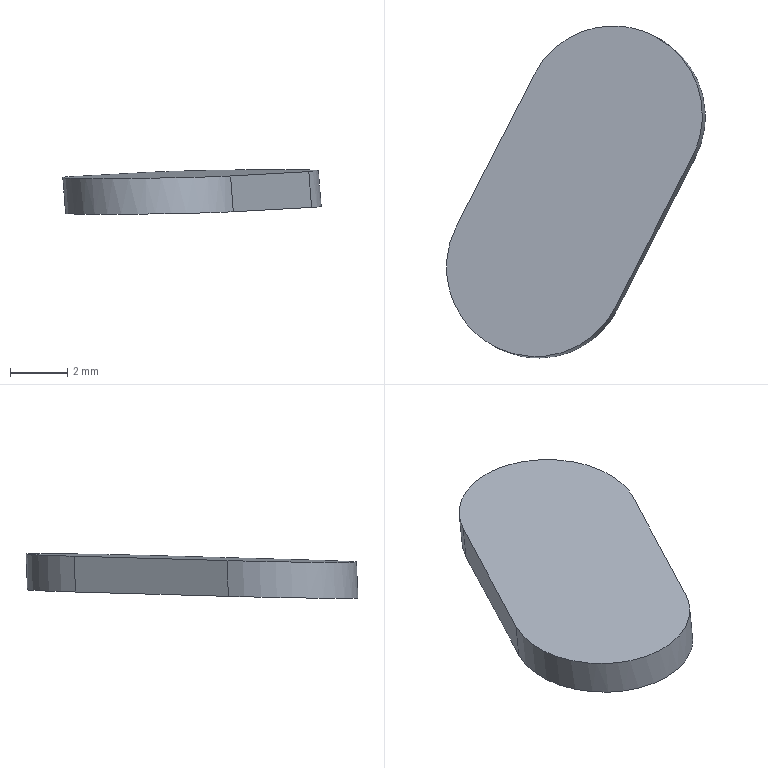Part | STEP file | gslz 2016.10.28-13_id1446_x_t | 1 solid | 6 faces | box 9.039 x 11.595 x 1.56 mm | volume 84.551 mm3 | plane 4 | cylinder 2 | commonest cylinder face diameters 6.2 x2
STEP:
#1=CARTESIAN_POINT('',(0.,0.,0.));
#2=DIRECTION('',(0.,0.,1.));
#3=DIRECTION('',(1.,0.,0.));
#4=AXIS2_PLACEMENT_3D('',#1,#2,#3);
#5=CARTESIAN_POINT('',(441.003,-201.542,-10.815));
#6=VERTEX_POINT('',#5);
#7=CARTESIAN_POINT('',(442.42,-205.757,-10.883));
#8=VERTEX_POINT('',#7);
#9=CARTESIAN_POINT('',(441.003,-201.542,-10.815));
#10=CARTESIAN_POINT('',(440.625,-202.28,-10.836));
#11=CARTESIAN_POINT('',(440.561,-203.16,-10.855));
#12=CARTESIAN_POINT('',(441.089,-204.728,-10.88));
#13=CARTESIAN_POINT('',(441.674,-205.394,-10.886));
#14=CARTESIAN_POINT('',(442.42,-205.757,-10.883));
#15=B_SPLINE_CURVE_WITH_KNOTS('',3,(#9,#10,#11,#12,#13,#14),.UNSPECIFIED.,.F.,.F.,(4,2,4),(0.,0.5,1.),.UNSPECIFIED.);
#16=CARTESIAN_POINT('',(447.998,-194.942,-10.575));
#17=DIRECTION('',(0.01446,0.021,-0.9997));
#18=DIRECTION('',(0.,0.9998,0.021));
#19=AXIS2_PLACEMENT_3D('',#16,#17,#18);
#20=PLANE('',#19);
#21=CARTESIAN_POINT('',(-6.604,-6.996));
#22=CARTESIAN_POINT('',(-7.342,-7.374));
#23=CARTESIAN_POINT('',(-8.223,-7.438));
#24=CARTESIAN_POINT('',(-9.791,-6.91));
#25=CARTESIAN_POINT('',(-10.457,-6.325));
#26=CARTESIAN_POINT('',(-10.82,-5.579));
#27=B_SPLINE_CURVE_WITH_KNOTS('',3,(#21,#22,#23,#24,#25,#26),.UNSPECIFIED.,.F.,.F.,(4,2,4),(0.,0.5,1.),.UNSPECIFIED.);
#28=(GEOMETRIC_REPRESENTATION_CONTEXT(2)PARAMETRIC_REPRESENTATION_CONTEXT()REPRESENTATION_CONTEXT('',''));
#29=DEFINITIONAL_REPRESENTATION('',(#27),#28);
#30=PCURVE('',#20,#29);
#31=CARTESIAN_POINT('',(443.763,-202.963,-10.73));
#32=DIRECTION('',(-0.07766,0.03957,0.9962));
#33=DIRECTION('',(-0.8876,0.4523,-0.08716));
#34=AXIS2_PLACEMENT_3D('',#31,#32,#33);
#35=CYLINDRICAL_SURFACE('',#34,3.1);
#36=CARTESIAN_POINT('',(-0.004096,0.186));
#37=CARTESIAN_POINT('',(1.59,-0.1586));
#38=B_SPLINE_CURVE_WITH_KNOTS('',1,(#36,#37),.UNSPECIFIED.,.F.,.F.,(2,2),(0.00000002,1.),.PIECEWISE_BEZIER_KNOTS.);
#39=(GEOMETRIC_REPRESENTATION_CONTEXT(2)PARAMETRIC_REPRESENTATION_CONTEXT()REPRESENTATION_CONTEXT('',''));
#40=DEFINITIONAL_REPRESENTATION('',(#38),#39);
#41=PCURVE('',#35,#40);
#42=SURFACE_CURVE('',#15,(#30,#41),.PCURVE_S1.);
#43=EDGE_CURVE('',#6,#8,#42,.T.);
#44=ORIENTED_EDGE('',*,*,#43,.T.);
#45=CARTESIAN_POINT('',(446.535,-204.39,-10.794));
#46=VERTEX_POINT('',#45);
#47=CARTESIAN_POINT('',(442.42,-205.757,-10.883));
#48=CARTESIAN_POINT('',(443.146,-206.11,-10.88));
#49=CARTESIAN_POINT('',(443.999,-206.166,-10.868));
#50=CARTESIAN_POINT('',(445.52,-205.66,-10.836));
#51=CARTESIAN_POINT('',(446.169,-205.104,-10.815));
#52=CARTESIAN_POINT('',(446.535,-204.39,-10.794));
#53=B_SPLINE_CURVE_WITH_KNOTS('',3,(#47,#48,#49,#50,#51,#52),.UNSPECIFIED.,.F.,.F.,(4,2,4),(0.,0.5,1.),.UNSPECIFIED.);
#54=CARTESIAN_POINT('',(-10.82,-5.579));
#55=CARTESIAN_POINT('',(-11.172,-4.853));
#56=CARTESIAN_POINT('',(-11.228,-3.999));
#57=CARTESIAN_POINT('',(-10.721,-2.479));
#58=CARTESIAN_POINT('',(-10.165,-1.83));
#59=CARTESIAN_POINT('',(-9.45,-1.464));
#60=B_SPLINE_CURVE_WITH_KNOTS('',3,(#54,#55,#56,#57,#58,#59),.UNSPECIFIED.,.F.,.F.,(4,2,4),(0.,0.5,1.),.UNSPECIFIED.);
#61=(GEOMETRIC_REPRESENTATION_CONTEXT(2)PARAMETRIC_REPRESENTATION_CONTEXT()REPRESENTATION_CONTEXT('',''));
#62=DEFINITIONAL_REPRESENTATION('',(#60),#61);
#63=PCURVE('',#20,#62);
#64=CARTESIAN_POINT('',(1.59,-0.1586));
#65=CARTESIAN_POINT('',(1.613,-0.1648));
#66=CARTESIAN_POINT('',(1.66,-0.1768));
#67=CARTESIAN_POINT('',(1.731,-0.1944));
#68=CARTESIAN_POINT('',(1.801,-0.2113));
#69=CARTESIAN_POINT('',(1.872,-0.2275));
#70=CARTESIAN_POINT('',(1.942,-0.243));
#71=CARTESIAN_POINT('',(2.012,-0.2576));
#72=CARTESIAN_POINT('',(2.082,-0.2714));
#73=CARTESIAN_POINT('',(2.153,-0.2842));
#74=CARTESIAN_POINT('',(2.223,-0.296));
#75=CARTESIAN_POINT('',(2.293,-0.3067));
#76=CARTESIAN_POINT('',(2.364,-0.3162));
#77=CARTESIAN_POINT('',(2.434,-0.3246));
#78=CARTESIAN_POINT('',(2.504,-0.3316));
#79=CARTESIAN_POINT('',(2.575,-0.3374));
#80=CARTESIAN_POINT('',(2.645,-0.3418));
#81=CARTESIAN_POINT('',(2.715,-0.345));
#82=CARTESIAN_POINT('',(2.785,-0.3469));
#83=CARTESIAN_POINT('',(2.856,-0.3475));
#84=CARTESIAN_POINT('',(2.926,-0.3467));
#85=CARTESIAN_POINT('',(2.996,-0.3446));
#86=CARTESIAN_POINT('',(3.067,-0.3412));
#87=CARTESIAN_POINT('',(3.114,-0.338));
#88=CARTESIAN_POINT('',(3.137,-0.3362));
#89=B_SPLINE_CURVE_WITH_KNOTS('',3,(#64,#65,#66,#67,#68,#69,#70,#71,#72,#73,#74,#75,#76,#77,#78,#79,#80,#81,#82,#83,#84,#85,#86,#87,#88),.UNSPECIFIED.,.F.,.F.,(4,1,1,1,1,1,1,1,1,1,1,1,1,1,1,1,1,1,1,1,1,1,4),(0.,0.04545,0.09091,0.1364,0.1818,0.2273,0.2727,0.3182,0.3636,0.4091,0.4545,0.5,0.5455,0.5909,0.6364,0.6818,0.7273,0.7727,0.8182,0.8636,0.9091,0.9545,1.),.QUASI_UNIFORM_KNOTS.);
#90=(GEOMETRIC_REPRESENTATION_CONTEXT(2)PARAMETRIC_REPRESENTATION_CONTEXT()REPRESENTATION_CONTEXT('',''));
#91=DEFINITIONAL_REPRESENTATION('',(#89),#90);
#92=PCURVE('',#35,#91);
#93=SURFACE_CURVE('',#53,(#63,#92),.PCURVE_S1.);
#94=EDGE_CURVE('',#8,#46,#93,.T.);
#95=ORIENTED_EDGE('',*,*,#94,.T.);
#96=CARTESIAN_POINT('',(449.269,-199.049,-10.643));
#97=VERTEX_POINT('',#96);
#98=CARTESIAN_POINT('',(449.269,-199.049,-10.643));
#99=DIRECTION('',(0.4555,0.8899,0.02528));
#100=VECTOR('',#99,1.);
#101=LINE('',#98,#100);
#102=CARTESIAN_POINT('',(-4.107,1.271));
#103=DIRECTION('',(0.8902,0.4556));
#104=VECTOR('',#103,1.);
#105=LINE('',#102,#104);
#106=(GEOMETRIC_REPRESENTATION_CONTEXT(2)PARAMETRIC_REPRESENTATION_CONTEXT()REPRESENTATION_CONTEXT('',''));
#107=DEFINITIONAL_REPRESENTATION('',(#105),#106);
#108=PCURVE('',#20,#107);
#109=CARTESIAN_POINT('',(449.254,-199.041,-10.457));
#110=DIRECTION('',(0.8857,-0.4559,0.08716));
#111=DIRECTION('',(-0.4576,-0.8891,-0.000357));
#112=AXIS2_PLACEMENT_3D('',#109,#110,#111);
#113=PLANE('',#112);
#114=CARTESIAN_POINT('',(0.,0.186));
#115=DIRECTION('',(-0.9997,-0.02502));
#116=VECTOR('',#115,1.);
#117=LINE('',#114,#116);
#118=(GEOMETRIC_REPRESENTATION_CONTEXT(2)PARAMETRIC_REPRESENTATION_CONTEXT()REPRESENTATION_CONTEXT('',''));
#119=DEFINITIONAL_REPRESENTATION('',(#117),#118);
#120=PCURVE('',#113,#119);
#121=SURFACE_CURVE('',#101,(#108,#120),.PCURVE_S1.);
#122=EDGE_CURVE('',#46,#97,#121,.T.);
#123=ORIENTED_EDGE('',*,*,#122,.T.);
#124=CARTESIAN_POINT('',(447.979,-194.899,-10.574));
#125=VERTEX_POINT('',#124);
#126=CARTESIAN_POINT('',(447.979,-194.899,-10.574));
#127=CARTESIAN_POINT('',(448.683,-195.282,-10.572));
#128=CARTESIAN_POINT('',(449.229,-195.947,-10.578));
#129=CARTESIAN_POINT('',(449.706,-197.478,-10.603));
#130=CARTESIAN_POINT('',(449.634,-198.335,-10.622));
#131=CARTESIAN_POINT('',(449.269,-199.049,-10.643));
#132=B_SPLINE_CURVE_WITH_KNOTS('',3,(#126,#127,#128,#129,#130,#131),.UNSPECIFIED.,.F.,.F.,(4,2,4),(0.,0.5,1.),.UNSPECIFIED.);
#133=CARTESIAN_POINT('',(0.04275,-0.01983));
#134=CARTESIAN_POINT('',(-0.3402,0.6846));
#135=CARTESIAN_POINT('',(-1.005,1.231));
#136=CARTESIAN_POINT('',(-2.536,1.708));
#137=CARTESIAN_POINT('',(-3.394,1.636));
#138=CARTESIAN_POINT('',(-4.107,1.271));
#139=B_SPLINE_CURVE_WITH_KNOTS('',3,(#133,#134,#135,#136,#137,#138),.UNSPECIFIED.,.F.,.F.,(4,2,4),(0.,0.5,1.),.UNSPECIFIED.);
#140=(GEOMETRIC_REPRESENTATION_CONTEXT(2)PARAMETRIC_REPRESENTATION_CONTEXT()REPRESENTATION_CONTEXT('',''));
#141=DEFINITIONAL_REPRESENTATION('',(#139),#140);
#142=PCURVE('',#20,#141);
#143=CARTESIAN_POINT('',(446.509,-197.628,-10.728));
#144=DIRECTION('',(-0.07766,0.03957,0.9962));
#145=DIRECTION('',(-0.8876,0.4523,-0.08716));
#146=AXIS2_PLACEMENT_3D('',#143,#144,#145);
#147=CYLINDRICAL_SURFACE('',#146,3.1);
#148=CARTESIAN_POINT('',(4.685,0.1467));
#149=CARTESIAN_POINT('',(3.137,-0.186));
#150=B_SPLINE_CURVE_WITH_KNOTS('',1,(#148,#149),.UNSPECIFIED.,.F.,.F.,(2,2),(0.,1.),.PIECEWISE_BEZIER_KNOTS.);
#151=(GEOMETRIC_REPRESENTATION_CONTEXT(2)PARAMETRIC_REPRESENTATION_CONTEXT()REPRESENTATION_CONTEXT('',''));
#152=DEFINITIONAL_REPRESENTATION('',(#150),#151);
#153=PCURVE('',#147,#152);
#154=SURFACE_CURVE('',#132,(#142,#153),.PCURVE_S1.);
#155=EDGE_CURVE('',#125,#97,#154,.T.);
#156=ORIENTED_EDGE('',*,*,#155,.F.);
#157=CARTESIAN_POINT('',(443.737,-196.201,-10.663));
#158=VERTEX_POINT('',#157);
#159=CARTESIAN_POINT('',(443.737,-196.201,-10.663));
#160=CARTESIAN_POINT('',(444.112,-195.468,-10.642));
#161=CARTESIAN_POINT('',(444.794,-194.897,-10.62));
#162=CARTESIAN_POINT('',(446.37,-194.414,-10.587));
#163=CARTESIAN_POINT('',(447.254,-194.505,-10.576));
#164=CARTESIAN_POINT('',(447.979,-194.899,-10.574));
#165=B_SPLINE_CURVE_WITH_KNOTS('',3,(#159,#160,#161,#162,#163,#164),.UNSPECIFIED.,.F.,.F.,(4,2,4),(0.,0.5,1.),.UNSPECIFIED.);
#166=CARTESIAN_POINT('',(-1.261,-4.262));
#167=CARTESIAN_POINT('',(-0.5273,-3.886));
#168=CARTESIAN_POINT('',(0.04373,-3.205));
#169=CARTESIAN_POINT('',(0.5269,-1.628));
#170=CARTESIAN_POINT('',(0.4366,-0.7442));
#171=CARTESIAN_POINT('',(0.04275,-0.01983));
#172=B_SPLINE_CURVE_WITH_KNOTS('',3,(#166,#167,#168,#169,#170,#171),.UNSPECIFIED.,.F.,.F.,(4,2,4),(0.,0.5,1.),.UNSPECIFIED.);
#173=(GEOMETRIC_REPRESENTATION_CONTEXT(2)PARAMETRIC_REPRESENTATION_CONTEXT()REPRESENTATION_CONTEXT('',''));
#174=DEFINITIONAL_REPRESENTATION('',(#172),#173);
#175=PCURVE('',#20,#174);
#176=CARTESIAN_POINT('',(6.279,0.3362));
#177=CARTESIAN_POINT('',(6.255,0.338));
#178=CARTESIAN_POINT('',(6.207,0.3413));
#179=CARTESIAN_POINT('',(6.134,0.3448));
#180=CARTESIAN_POINT('',(6.062,0.3468));
#181=CARTESIAN_POINT('',(5.989,0.3474));
#182=CARTESIAN_POINT('',(5.916,0.3466));
#183=CARTESIAN_POINT('',(5.844,0.3445));
#184=CARTESIAN_POINT('',(5.771,0.3409));
#185=CARTESIAN_POINT('',(5.699,0.336));
#186=CARTESIAN_POINT('',(5.626,0.3297));
#187=CARTESIAN_POINT('',(5.554,0.3221));
#188=CARTESIAN_POINT('',(5.481,0.3132));
#189=CARTESIAN_POINT('',(5.409,0.3029));
#190=CARTESIAN_POINT('',(5.337,0.2914));
#191=CARTESIAN_POINT('',(5.264,0.2788));
#192=CARTESIAN_POINT('',(5.192,0.2651));
#193=CARTESIAN_POINT('',(5.119,0.2505));
#194=CARTESIAN_POINT('',(5.047,0.235));
#195=CARTESIAN_POINT('',(4.975,0.2186));
#196=CARTESIAN_POINT('',(4.902,0.2015));
#197=CARTESIAN_POINT('',(4.83,0.1838));
#198=CARTESIAN_POINT('',(4.758,0.1655));
#199=CARTESIAN_POINT('',(4.709,0.153));
#200=CARTESIAN_POINT('',(4.685,0.1467));
#201=B_SPLINE_CURVE_WITH_KNOTS('',3,(#176,#177,#178,#179,#180,#181,#182,#183,#184,#185,#186,#187,#188,#189,#190,#191,#192,#193,#194,#195,#196,#197,#198,#199,#200),.UNSPECIFIED.,.F.,.F.,(4,1,1,1,1,1,1,1,1,1,1,1,1,1,1,1,1,1,1,1,1,1,4),(0.00000002,0.04545,0.09091,0.1364,0.1818,0.2273,0.2727,0.3182,0.3636,0.4091,0.4545,0.5,0.5455,0.5909,0.6364,0.6818,0.7273,0.7727,0.8182,0.8636,0.9091,0.9545,1.),.QUASI_UNIFORM_KNOTS.);
#202=(GEOMETRIC_REPRESENTATION_CONTEXT(2)PARAMETRIC_REPRESENTATION_CONTEXT()REPRESENTATION_CONTEXT('',''));
#203=DEFINITIONAL_REPRESENTATION('',(#201),#202);
#204=PCURVE('',#147,#203);
#205=SURFACE_CURVE('',#165,(#175,#204),.PCURVE_S1.);
#206=EDGE_CURVE('',#158,#125,#205,.T.);
#207=ORIENTED_EDGE('',*,*,#206,.F.);
#208=CARTESIAN_POINT('',(445.133,-193.474,-10.585));
#209=DIRECTION('',(0.4555,0.8899,0.02528));
#210=VECTOR('',#209,1.);
#211=LINE('',#208,#210);
#212=CARTESIAN_POINT('',(1.467,-2.866));
#213=DIRECTION('',(0.8902,0.4556));
#214=VECTOR('',#213,1.);
#215=LINE('',#212,#214);
#216=(GEOMETRIC_REPRESENTATION_CONTEXT(2)PARAMETRIC_REPRESENTATION_CONTEXT()REPRESENTATION_CONTEXT('',''));
#217=DEFINITIONAL_REPRESENTATION('',(#215),#216);
#218=PCURVE('',#20,#217);
#219=CARTESIAN_POINT('',(441.017,-201.55,-11.));
#220=DIRECTION('',(-0.8857,0.4559,-0.08716));
#221=DIRECTION('',(0.4576,0.8891,0.000357));
#222=AXIS2_PLACEMENT_3D('',#219,#220,#221);
#223=PLANE('',#222);
#224=CARTESIAN_POINT('',(9.063,-0.4128));
#225=DIRECTION('',(0.9997,-0.02502));
#226=VECTOR('',#225,1.);
#227=LINE('',#224,#226);
#228=(GEOMETRIC_REPRESENTATION_CONTEXT(2)PARAMETRIC_REPRESENTATION_CONTEXT()REPRESENTATION_CONTEXT('',''));
#229=DEFINITIONAL_REPRESENTATION('',(#227),#228);
#230=PCURVE('',#223,#229);
#231=SURFACE_CURVE('',#211,(#218,#230),.PCURVE_S1.);
#232=EDGE_CURVE('',#6,#158,#231,.T.);
#233=ORIENTED_EDGE('',*,*,#232,.F.);
#234=EDGE_LOOP('',(#44,#95,#123,#156,#207,#233));
#235=FACE_BOUND('',#234,.T.);
#236=ADVANCED_FACE('',(#235),#20,.F.);
#237=CARTESIAN_POINT('',(446.632,-204.439,-12.044));
#238=VERTEX_POINT('',#237);
#239=CARTESIAN_POINT('',(446.509,-204.376,-10.46));
#240=DIRECTION('',(-0.07766,0.03957,0.9962));
#241=VECTOR('',#240,1.);
#242=LINE('',#239,#241);
#243=CARTESIAN_POINT('',(3.137,0.));
#244=DIRECTION('',(0.,1.));
#245=VECTOR('',#244,1.);
#246=LINE('',#243,#245);
#247=(GEOMETRIC_REPRESENTATION_CONTEXT(2)PARAMETRIC_REPRESENTATION_CONTEXT()REPRESENTATION_CONTEXT('',''));
#248=DEFINITIONAL_REPRESENTATION('',(#246),#247);
#249=PCURVE('',#35,#248);
#250=CARTESIAN_POINT('',(6.,0.));
#251=DIRECTION('',(0.,-1.));
#252=VECTOR('',#251,1.);
#253=LINE('',#250,#252);
#254=(GEOMETRIC_REPRESENTATION_CONTEXT(2)PARAMETRIC_REPRESENTATION_CONTEXT()REPRESENTATION_CONTEXT('',''));
#255=DEFINITIONAL_REPRESENTATION('',(#253),#254);
#256=PCURVE('',#113,#255);
#257=SURFACE_CURVE('',#242,(#249,#256),.PCURVE_S1.);
#258=EDGE_CURVE('',#238,#46,#257,.T.);
#259=ORIENTED_EDGE('',*,*,#258,.T.);
#260=ORIENTED_EDGE('',*,*,#94,.F.);
#261=ORIENTED_EDGE('',*,*,#43,.F.);
#262=CARTESIAN_POINT('',(441.1,-201.592,-12.065));
#263=VERTEX_POINT('',#262);
#264=CARTESIAN_POINT('',(441.017,-201.55,-11.));
#265=DIRECTION('',(-0.07766,0.03957,0.9962));
#266=VECTOR('',#265,1.);
#267=LINE('',#264,#266);
#268=CARTESIAN_POINT('',(-0.004096,0.));
#269=DIRECTION('',(0.,1.));
#270=VECTOR('',#269,1.);
#271=LINE('',#268,#270);
#272=(GEOMETRIC_REPRESENTATION_CONTEXT(2)PARAMETRIC_REPRESENTATION_CONTEXT()REPRESENTATION_CONTEXT('',''));
#273=DEFINITIONAL_REPRESENTATION('',(#271),#272);
#274=PCURVE('',#35,#273);
#275=CARTESIAN_POINT('',(0.,0.));
#276=DIRECTION('',(0.,-1.));
#277=VECTOR('',#276,1.);
#278=LINE('',#275,#277);
#279=(GEOMETRIC_REPRESENTATION_CONTEXT(2)PARAMETRIC_REPRESENTATION_CONTEXT()REPRESENTATION_CONTEXT('',''));
#280=DEFINITIONAL_REPRESENTATION('',(#278),#279);
#281=PCURVE('',#223,#280);
#282=SURFACE_CURVE('',#267,(#274,#281),.PCURVE_S1.);
#283=EDGE_CURVE('',#263,#6,#282,.T.);
#284=ORIENTED_EDGE('',*,*,#283,.F.);
#285=CARTESIAN_POINT('',(441.1,-201.592,-12.065));
#286=CARTESIAN_POINT('',(440.73,-202.315,-12.085));
#287=CARTESIAN_POINT('',(440.661,-203.187,-12.105));
#288=CARTESIAN_POINT('',(441.162,-204.734,-12.13));
#289=CARTESIAN_POINT('',(441.728,-205.401,-12.136));
#290=CARTESIAN_POINT('',(443.173,-206.146,-12.13));
#291=CARTESIAN_POINT('',(444.045,-206.221,-12.119));
#292=CARTESIAN_POINT('',(445.594,-205.728,-12.087));
#293=CARTESIAN_POINT('',(446.262,-205.163,-12.065));
#294=CARTESIAN_POINT('',(446.632,-204.439,-12.044));
#295=B_SPLINE_CURVE_WITH_KNOTS('',3,(#285,#286,#287,#288,#289,#290,#291,#292,#293,#294),.UNSPECIFIED.,.F.,.F.,(4,2,2,2,4),(0.,0.25,0.5,0.75,1.),.UNSPECIFIED.);
#296=CARTESIAN_POINT('',(-0.004096,-1.069));
#297=CARTESIAN_POINT('',(0.04355,-1.073));
#298=CARTESIAN_POINT('',(0.1388,-1.082));
#299=CARTESIAN_POINT('',(0.2817,-1.101));
#300=CARTESIAN_POINT('',(0.4247,-1.124));
#301=CARTESIAN_POINT('',(0.5676,-1.152));
#302=CARTESIAN_POINT('',(0.7103,-1.183));
#303=CARTESIAN_POINT('',(0.8529,-1.217));
#304=CARTESIAN_POINT('',(0.9954,-1.254));
#305=CARTESIAN_POINT('',(1.138,-1.292));
#306=CARTESIAN_POINT('',(1.281,-1.331));
#307=CARTESIAN_POINT('',(1.423,-1.369));
#308=CARTESIAN_POINT('',(1.566,-1.407));
#309=CARTESIAN_POINT('',(1.708,-1.444));
#310=CARTESIAN_POINT('',(1.851,-1.478));
#311=CARTESIAN_POINT('',(1.994,-1.509));
#312=CARTESIAN_POINT('',(2.137,-1.537));
#313=CARTESIAN_POINT('',(2.279,-1.56));
#314=CARTESIAN_POINT('',(2.422,-1.579));
#315=CARTESIAN_POINT('',(2.565,-1.592));
#316=CARTESIAN_POINT('',(2.708,-1.6));
#317=CARTESIAN_POINT('',(2.851,-1.603));
#318=CARTESIAN_POINT('',(2.995,-1.6));
#319=CARTESIAN_POINT('',(3.09,-1.595));
#320=CARTESIAN_POINT('',(3.137,-1.591));
#321=B_SPLINE_CURVE_WITH_KNOTS('',3,(#296,#297,#298,#299,#300,#301,#302,#303,#304,#305,#306,#307,#308,#309,#310,#311,#312,#313,#314,#315,#316,#317,#318,#319,#320),.UNSPECIFIED.,.F.,.F.,(4,1,1,1,1,1,1,1,1,1,1,1,1,1,1,1,1,1,1,1,1,1,4),(0.,0.04545,0.09091,0.1364,0.1818,0.2273,0.2727,0.3182,0.3636,0.4091,0.4545,0.5,0.5455,0.5909,0.6364,0.6818,0.7273,0.7727,0.8182,0.8636,0.9091,0.9545,1.),.QUASI_UNIFORM_KNOTS.);
#322=(GEOMETRIC_REPRESENTATION_CONTEXT(2)PARAMETRIC_REPRESENTATION_CONTEXT()REPRESENTATION_CONTEXT('',''));
#323=DEFINITIONAL_REPRESENTATION('',(#321),#322);
#324=PCURVE('',#35,#323);
#325=CARTESIAN_POINT('',(448.016,-194.916,-11.824));
#326=DIRECTION('',(0.01446,0.021,-0.9997));
#327=DIRECTION('',(0.,0.9998,0.021));
#328=AXIS2_PLACEMENT_3D('',#325,#326,#327);
#329=PLANE('',#328);
#330=CARTESIAN_POINT('',(-6.68,-6.917));
#331=CARTESIAN_POINT('',(-7.404,-7.288));
#332=CARTESIAN_POINT('',(-8.276,-7.356));
#333=CARTESIAN_POINT('',(-9.823,-6.855));
#334=CARTESIAN_POINT('',(-10.489,-6.289));
#335=CARTESIAN_POINT('',(-11.235,-4.844));
#336=CARTESIAN_POINT('',(-11.309,-3.972));
#337=CARTESIAN_POINT('',(-10.816,-2.423));
#338=CARTESIAN_POINT('',(-10.25,-1.755));
#339=CARTESIAN_POINT('',(-9.526,-1.384));
#340=B_SPLINE_CURVE_WITH_KNOTS('',3,(#330,#331,#332,#333,#334,#335,#336,#337,#338,#339),.UNSPECIFIED.,.F.,.F.,(4,2,2,2,4),(0.,0.25,0.5,0.75,1.),.UNSPECIFIED.);
#341=(GEOMETRIC_REPRESENTATION_CONTEXT(2)PARAMETRIC_REPRESENTATION_CONTEXT()REPRESENTATION_CONTEXT('',''));
#342=DEFINITIONAL_REPRESENTATION('',(#340),#341);
#343=PCURVE('',#329,#342);
#344=SURFACE_CURVE('',#295,(#324,#343),.PCURVE_S1.);
#345=EDGE_CURVE('',#263,#238,#344,.T.);
#346=ORIENTED_EDGE('',*,*,#345,.T.);
#347=EDGE_LOOP('',(#259,#260,#261,#284,#346));
#348=FACE_BOUND('',#347,.T.);
#349=ADVANCED_FACE('',(#348),#35,.T.);
#350=ORIENTED_EDGE('',*,*,#283,.T.);
#351=ORIENTED_EDGE('',*,*,#232,.T.);
#352=CARTESIAN_POINT('',(443.834,-196.251,-11.913));
#353=VERTEX_POINT('',#352);
#354=CARTESIAN_POINT('',(443.763,-196.215,-10.998));
#355=DIRECTION('',(-0.07766,0.03957,0.9962));
#356=VECTOR('',#355,1.);
#357=LINE('',#354,#356);
#358=CARTESIAN_POINT('',(6.,0.));
#359=DIRECTION('',(0.,-1.));
#360=VECTOR('',#359,1.);
#361=LINE('',#358,#360);
#362=(GEOMETRIC_REPRESENTATION_CONTEXT(2)PARAMETRIC_REPRESENTATION_CONTEXT()REPRESENTATION_CONTEXT('',''));
#363=DEFINITIONAL_REPRESENTATION('',(#361),#362);
#364=PCURVE('',#223,#363);
#365=CARTESIAN_POINT('',(6.279,0.));
#366=DIRECTION('',(0.,1.));
#367=VECTOR('',#366,1.);
#368=LINE('',#365,#367);
#369=(GEOMETRIC_REPRESENTATION_CONTEXT(2)PARAMETRIC_REPRESENTATION_CONTEXT()REPRESENTATION_CONTEXT('',''));
#370=DEFINITIONAL_REPRESENTATION('',(#368),#369);
#371=PCURVE('',#147,#370);
#372=SURFACE_CURVE('',#357,(#364,#371),.PCURVE_S1.);
#373=EDGE_CURVE('',#353,#158,#372,.T.);
#374=ORIENTED_EDGE('',*,*,#373,.F.);
#375=CARTESIAN_POINT('',(443.834,-196.251,-11.913));
#376=DIRECTION('',(0.4555,0.8899,0.02528));
#377=VECTOR('',#376,1.);
#378=LINE('',#375,#377);
#379=CARTESIAN_POINT('',(6.,0.9187));
#380=DIRECTION('',(0.9997,-0.02502));
#381=VECTOR('',#380,1.);
#382=LINE('',#379,#381);
#383=(GEOMETRIC_REPRESENTATION_CONTEXT(2)PARAMETRIC_REPRESENTATION_CONTEXT()REPRESENTATION_CONTEXT('',''));
#384=DEFINITIONAL_REPRESENTATION('',(#382),#383);
#385=PCURVE('',#223,#384);
#386=CARTESIAN_POINT('',(-1.337,-4.183));
#387=DIRECTION('',(0.8902,0.4556));
#388=VECTOR('',#387,1.);
#389=LINE('',#386,#388);
#390=(GEOMETRIC_REPRESENTATION_CONTEXT(2)PARAMETRIC_REPRESENTATION_CONTEXT()REPRESENTATION_CONTEXT('',''));
#391=DEFINITIONAL_REPRESENTATION('',(#389),#390);
#392=PCURVE('',#329,#391);
#393=SURFACE_CURVE('',#378,(#385,#392),.PCURVE_S1.);
#394=EDGE_CURVE('',#263,#353,#393,.T.);
#395=ORIENTED_EDGE('',*,*,#394,.F.);
#396=EDGE_LOOP('',(#350,#351,#374,#395));
#397=FACE_BOUND('',#396,.T.);
#398=ADVANCED_FACE('',(#397),#223,.T.);
#399=CARTESIAN_POINT('',(449.366,-199.098,-11.893));
#400=VERTEX_POINT('',#399);
#401=CARTESIAN_POINT('',(449.254,-199.041,-10.457));
#402=DIRECTION('',(-0.07766,0.03957,0.9962));
#403=VECTOR('',#402,1.);
#404=LINE('',#401,#403);
#405=CARTESIAN_POINT('',(0.,0.));
#406=DIRECTION('',(0.,-1.));
#407=VECTOR('',#406,1.);
#408=LINE('',#405,#407);
#409=(GEOMETRIC_REPRESENTATION_CONTEXT(2)PARAMETRIC_REPRESENTATION_CONTEXT()REPRESENTATION_CONTEXT('',''));
#410=DEFINITIONAL_REPRESENTATION('',(#408),#409);
#411=PCURVE('',#113,#410);
#412=CARTESIAN_POINT('',(3.137,0.));
#413=DIRECTION('',(0.,1.));
#414=VECTOR('',#413,1.);
#415=LINE('',#412,#414);
#416=(GEOMETRIC_REPRESENTATION_CONTEXT(2)PARAMETRIC_REPRESENTATION_CONTEXT()REPRESENTATION_CONTEXT('',''));
#417=DEFINITIONAL_REPRESENTATION('',(#415),#416);
#418=PCURVE('',#147,#417);
#419=SURFACE_CURVE('',#404,(#411,#418),.PCURVE_S1.);
#420=EDGE_CURVE('',#400,#97,#419,.T.);
#421=ORIENTED_EDGE('',*,*,#420,.T.);
#422=ORIENTED_EDGE('',*,*,#122,.F.);
#423=ORIENTED_EDGE('',*,*,#258,.F.);
#424=CARTESIAN_POINT('',(449.383,-199.066,-11.892));
#425=DIRECTION('',(0.4555,0.8899,0.02528));
#426=VECTOR('',#425,1.);
#427=LINE('',#424,#426);
#428=CARTESIAN_POINT('',(-0.03604,1.44));
#429=DIRECTION('',(-0.9997,-0.02502));
#430=VECTOR('',#429,1.);
#431=LINE('',#428,#430);
#432=(GEOMETRIC_REPRESENTATION_CONTEXT(2)PARAMETRIC_REPRESENTATION_CONTEXT()REPRESENTATION_CONTEXT('',''));
#433=DEFINITIONAL_REPRESENTATION('',(#431),#432);
#434=PCURVE('',#113,#433);
#435=CARTESIAN_POINT('',(-4.151,1.366));
#436=DIRECTION('',(0.8902,0.4556));
#437=VECTOR('',#436,1.);
#438=LINE('',#435,#437);
#439=(GEOMETRIC_REPRESENTATION_CONTEXT(2)PARAMETRIC_REPRESENTATION_CONTEXT()REPRESENTATION_CONTEXT('',''));
#440=DEFINITIONAL_REPRESENTATION('',(#438),#439);
#441=PCURVE('',#329,#440);
#442=SURFACE_CURVE('',#427,(#434,#441),.PCURVE_S1.);
#443=EDGE_CURVE('',#238,#400,#442,.T.);
#444=ORIENTED_EDGE('',*,*,#443,.T.);
#445=EDGE_LOOP('',(#421,#422,#423,#444));
#446=FACE_BOUND('',#445,.T.);
#447=ADVANCED_FACE('',(#446),#113,.T.);
#448=ORIENTED_EDGE('',*,*,#373,.T.);
#449=ORIENTED_EDGE('',*,*,#206,.T.);
#450=ORIENTED_EDGE('',*,*,#155,.T.);
#451=ORIENTED_EDGE('',*,*,#420,.F.);
#452=CARTESIAN_POINT('',(443.834,-196.251,-11.913));
#453=CARTESIAN_POINT('',(444.207,-195.523,-11.892));
#454=CARTESIAN_POINT('',(444.871,-194.962,-11.871));
#455=CARTESIAN_POINT('',(446.423,-194.469,-11.838));
#456=CARTESIAN_POINT('',(447.292,-194.543,-11.827));
#457=CARTESIAN_POINT('',(448.74,-195.29,-11.822));
#458=CARTESIAN_POINT('',(449.304,-195.955,-11.828));
#459=CARTESIAN_POINT('',(449.805,-197.504,-11.853));
#460=CARTESIAN_POINT('',(449.738,-198.372,-11.872));
#461=CARTESIAN_POINT('',(449.366,-199.098,-11.893));
#462=B_SPLINE_CURVE_WITH_KNOTS('',3,(#452,#453,#454,#455,#456,#457,#458,#459,#460,#461),.UNSPECIFIED.,.F.,.F.,(4,2,2,2,4),(0.,0.25,0.5,0.75,1.),.UNSPECIFIED.);
#463=CARTESIAN_POINT('',(6.279,-0.9187));
#464=CARTESIAN_POINT('',(6.231,-0.9149));
#465=CARTESIAN_POINT('',(6.135,-0.9094));
#466=CARTESIAN_POINT('',(5.992,-0.9066));
#467=CARTESIAN_POINT('',(5.85,-0.9094));
#468=CARTESIAN_POINT('',(5.707,-0.9175));
#469=CARTESIAN_POINT('',(5.564,-0.9309));
#470=CARTESIAN_POINT('',(5.421,-0.9496));
#471=CARTESIAN_POINT('',(5.278,-0.973));
#472=CARTESIAN_POINT('',(5.135,-1.001));
#473=CARTESIAN_POINT('',(4.992,-1.032));
#474=CARTESIAN_POINT('',(4.85,-1.066));
#475=CARTESIAN_POINT('',(4.707,-1.102));
#476=CARTESIAN_POINT('',(4.565,-1.14));
#477=CARTESIAN_POINT('',(4.422,-1.179));
#478=CARTESIAN_POINT('',(4.28,-1.218));
#479=CARTESIAN_POINT('',(4.137,-1.256));
#480=CARTESIAN_POINT('',(3.995,-1.292));
#481=CARTESIAN_POINT('',(3.852,-1.327));
#482=CARTESIAN_POINT('',(3.709,-1.358));
#483=CARTESIAN_POINT('',(3.567,-1.385));
#484=CARTESIAN_POINT('',(3.424,-1.409));
#485=CARTESIAN_POINT('',(3.281,-1.428));
#486=CARTESIAN_POINT('',(3.185,-1.437));
#487=CARTESIAN_POINT('',(3.137,-1.441));
#488=B_SPLINE_CURVE_WITH_KNOTS('',3,(#463,#464,#465,#466,#467,#468,#469,#470,#471,#472,#473,#474,#475,#476,#477,#478,#479,#480,#481,#482,#483,#484,#485,#486,#487),.UNSPECIFIED.,.F.,.F.,(4,1,1,1,1,1,1,1,1,1,1,1,1,1,1,1,1,1,1,1,1,1,4),(0.,0.04545,0.09091,0.1364,0.1818,0.2273,0.2727,0.3182,0.3636,0.4091,0.4545,0.5,0.5455,0.5909,0.6364,0.6818,0.7273,0.7727,0.8182,0.8636,0.9091,0.9545,1.),.QUASI_UNIFORM_KNOTS.);
#489=(GEOMETRIC_REPRESENTATION_CONTEXT(2)PARAMETRIC_REPRESENTATION_CONTEXT()REPRESENTATION_CONTEXT('',''));
#490=DEFINITIONAL_REPRESENTATION('',(#488),#489);
#491=PCURVE('',#147,#490);
#492=CARTESIAN_POINT('',(-1.337,-4.183));
#493=CARTESIAN_POINT('',(-0.609,-3.81));
#494=CARTESIAN_POINT('',(-0.04782,-3.146));
#495=CARTESIAN_POINT('',(0.4463,-1.593));
#496=CARTESIAN_POINT('',(0.3722,-0.7245));
#497=CARTESIAN_POINT('',(-0.3747,0.7231));
#498=CARTESIAN_POINT('',(-1.039,1.288));
#499=CARTESIAN_POINT('',(-2.588,1.789));
#500=CARTESIAN_POINT('',(-3.457,1.722));
#501=CARTESIAN_POINT('',(-4.183,1.35));
#502=B_SPLINE_CURVE_WITH_KNOTS('',3,(#492,#493,#494,#495,#496,#497,#498,#499,#500,#501),.UNSPECIFIED.,.F.,.F.,(4,2,2,2,4),(0.,0.25,0.5,0.75,1.),.UNSPECIFIED.);
#503=(GEOMETRIC_REPRESENTATION_CONTEXT(2)PARAMETRIC_REPRESENTATION_CONTEXT()REPRESENTATION_CONTEXT('',''));
#504=DEFINITIONAL_REPRESENTATION('',(#502),#503);
#505=PCURVE('',#329,#504);
#506=SURFACE_CURVE('',#462,(#491,#505),.PCURVE_S1.);
#507=EDGE_CURVE('',#353,#400,#506,.T.);
#508=ORIENTED_EDGE('',*,*,#507,.F.);
#509=EDGE_LOOP('',(#448,#449,#450,#451,#508));
#510=FACE_BOUND('',#509,.T.);
#511=ADVANCED_FACE('',(#510),#147,.T.);
#512=ORIENTED_EDGE('',*,*,#507,.T.);
#513=ORIENTED_EDGE('',*,*,#443,.F.);
#514=ORIENTED_EDGE('',*,*,#345,.F.);
#515=ORIENTED_EDGE('',*,*,#394,.T.);
#516=EDGE_LOOP('',(#512,#513,#514,#515));
#517=FACE_BOUND('',#516,.T.);
#518=ADVANCED_FACE('',(#517),#329,.T.);
#519=CLOSED_SHELL('',(#236,#349,#398,#447,#511,#518));
#520=MANIFOLD_SOLID_BREP('',#519);
#521=(LENGTH_UNIT()NAMED_UNIT(*)SI_UNIT(.MILLI.,.METRE.));
#522=UNCERTAINTY_MEASURE_WITH_UNIT(LENGTH_MEASURE(0.01),#521,'','');
#523=(NAMED_UNIT(*)PLANE_ANGLE_UNIT()SI_UNIT($,.RADIAN.));
#524=(NAMED_UNIT(*)SI_UNIT($,.STERADIAN.)SOLID_ANGLE_UNIT());
#525=(GEOMETRIC_REPRESENTATION_CONTEXT(3)GLOBAL_UNCERTAINTY_ASSIGNED_CONTEXT((#522))GLOBAL_UNIT_ASSIGNED_CONTEXT((#521,#523,#524))REPRESENTATION_CONTEXT('',''));
#526=ADVANCED_BREP_SHAPE_REPRESENTATION('',(#4,#520),#525);